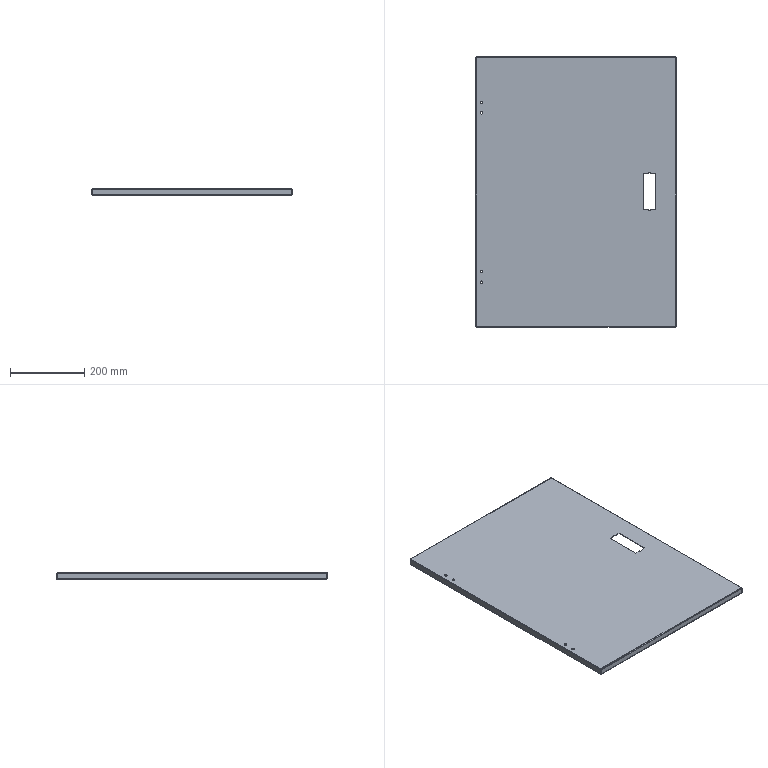Part | SolidWorks | features EdgeFlange 5, Cut 1, FlatPattern 1, ICE 1, SMBaseFlange 1, SheetMetal 1, WeldmentFeature 1 | 1 solid | 98 faces | box 539 x 728 x 18 mm | volume 690643 mm3 | plane 60 | cylinder 30 | spline 8 | commonest cylinder face diameters 6.5 x12 1.473 x8 4.473 x8 6 x2